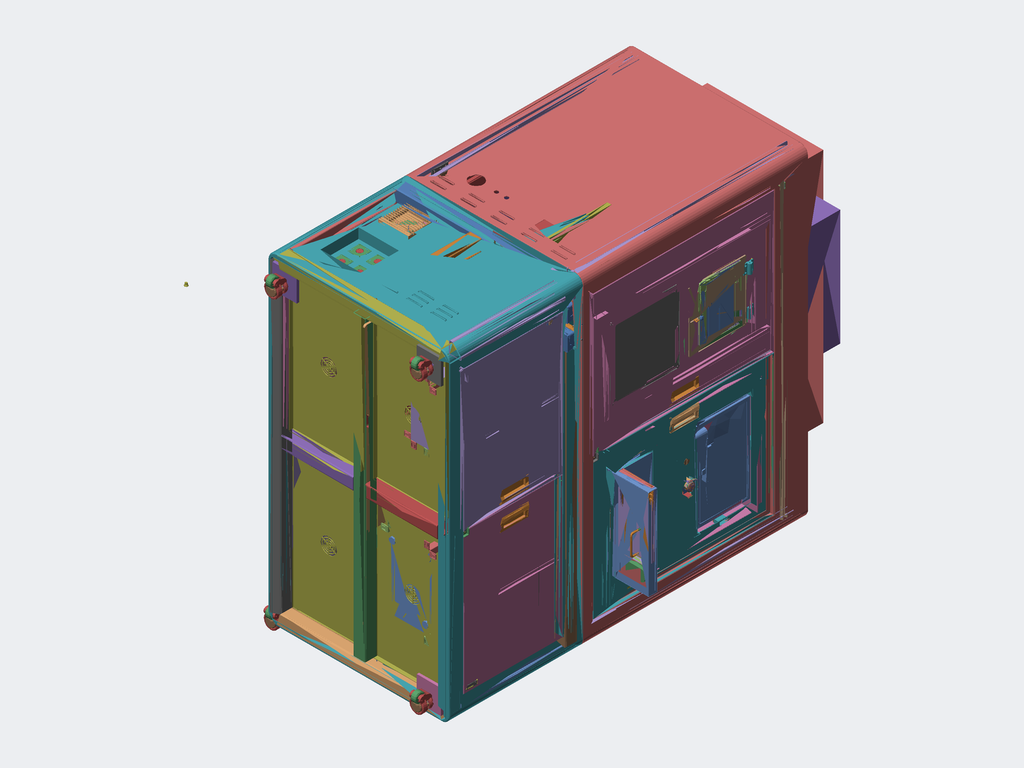Assembly | STEP file | 352 different items | 674 placed
Parts list (item | name | quantity | parent item | size | volume), first 270 of 352 items:
1 | Square tube frame_default<as machined> | x1 | in Lower frame | 896 x 660 x 1596 mm | 13190775 mm3
2 | Lower seal plate | x4 | in Lower frame | 708 x 358 x 20 mm | 574512 mm3
3 | ND25021-01-JDKM-103-TL | x1 | in Lower frame | 1490 x 15 x 786 mm | 17159345 mm3
4 | H_ND24021-01-JG-103-TL | x1 | in Lower frame | 1300 x 10 x 480 mm | 6236216 mm3
5 | PC | x1 | in Industrial PC assembly | 380 x 205 x 480 mm | 36265912 mm3
6 | PClimit part | x4 | in Industrial PC assembly, UPSassembly | 58 x 58 x 53 mm | 11788 mm3
7 | PC限位件2 | x4 | in Industrial PC assembly, UPSassembly | 58 x 58 x 53 mm | 11788 mm3
8 | Lower frame door panel | x2 | in Lower机架DoorPlate 2 | 20 x 700 x 502 mm | 890062 mm3
9 | HI_HFG87-17-001(2)^HFG87-17(2)_Lower机架DoorPlate 2 | x2 | in HFG87-17(2)^Lower机架DoorPlate 2 | 21.5 x 9 x 60 mm | 2771 mm3
10 | HI_HFG87-17-002(2)^HFG87-17(2)_Lower机架DoorPlate 2 | x2 | in HFG87-17(2)^Lower机架DoorPlate 2 | 18 x 8 x 84 mm | 2771 mm3
11 | XAM35_A140 | x7 | in Lower机架DoorPlate 2, 8, ND22021-MA-C-111, CE-005 | 64 x 22.5 x 140 mm | 66990 mm3
12 | OP02-QR01-J618 | x10 | in Door suction with buffer_9 | 27 x 27 x 12 mm | 2284 mm3
13 | Rubber buffer pad | x10 | in Door suction with buffer_9 | 22 x 22 x 7 mm | 750.57 mm3
14 | NHXCC20-5.5 | x10 | in Door suction with buffer_9 | 20 x 20 x 5.5 mm | 1502 mm3
15 | Flat-head stainless hex socket screw_M5_8 | x10 | in Door suction with buffer_9 | 10 x 10 x 11.1 mm | 211.569 mm3
16 | NNX210 | x2 | in 8 | 20 x 700 x 502 mm | 889755 mm3
17 | HI_HFG87-17-001(2)^ HFG87-17(2)_Lower frame door panel | x2 | in HFG87-17(2)^Lower frame door panel | 21.5 x 9 x 60 mm | 2771 mm3
18 | HI_HFG87-17-002(2)^ HFG87-17(2)_Lower frame door panel | x2 | in HFG87-17(2)^Lower frame door panel | 18 x 8 x 84 mm | 2771 mm3
19 | B-002 | x1 | in Lower frame | 1610 x 665 x 900 mm | 5357504 mm3
20 | with guard(8 mounting holes M5 metric threaded holes) Fan-KM | x2 | in Cooling Fanassembly-KM | - | -
21 | Ventilation filter assembly-KM | x2 | in Cooling Fanassembly-KM | 149 x 149 x 28 mm | 126448 mm3
22 | 电源1 | x1 | in Power switch | 105 x 85 x 79 mm | 30351 mm3
23 | 电源2 | x1 | in Power switch | 61 x 20 x 2 mm | 2336 mm3
24 | 电源3 | x1 | in Power switch | - | -
25 | AC20D-02C-A_0_^气源二联件-SMC | x1 | in 气源二联件-SMC | 83.2 x 172.3 x 53.4 mm | 301660 mm3
26 | _HSV08 -slide | x1 | in HSV08 | 30 x 30 x 32.5 mm | 8449 mm3
27 | _HSV08 Body | x1 | in HSV08 | 21.939 x 19.4 x 58 mm | 11797 mm3
28 | PL1002 | x2 | in 气源二联件-SMC | 35.315 x 36 x 18 mm | 6237 mm3
29 | ISE30A-01-N-ML_0_^气源二联件-SMC | x1 | in 气源二联件-SMC | 30 x 30 x 60.1 mm | 24209 mm3
30 | 接头6 | x2 | in Lower frame | 60 x 60 x 1.5 mm | 5253 mm3
31 | Ethernet port | x1 | in 接头3 | 60 x 60 x 1.5 mm | 5226 mm3
32 | 接头2 | x3 | in Lower frame | 60 x 60 x 1.5 mm | 5261 mm3
33 | UPS | x1 | in UPSassembly | 275 x 90 x 240 mm | 5940000 mm3
34 | H_ND24021-01-JG-098-TL | x1 | in power cover plate | 600 x 5 x 180 mm | 537768 mm3
35 | H_ND24021-01-JG-096-TL | x4 | in power cover plate | 43 x 20 x 132 mm | 6992 mm3
36 | HAU61-M5-L15^power cover plate | x4 | in power cover plate | 20 x 19.896 x 23 mm | 3201 mm3
37 | JK-Aviation plug | x4 | in Lower frame | 60 x 60 x 1.5 mm | 5200 mm3
38 | H_ND24021-01-JG-032-SL | x2 | in Air source cover plate | 300 x 5 x 255 mm | 380407 mm3
39 | HAQ07-M5^Air source cover plate | x2 | in Air source cover plate | 17 x 15 x 17 mm | 1673 mm3
40 | H_ND24021-01-JG-029-BJ | x3 | in Air source cover plate | 25.5 x 30 x 17.5 mm | 1036 mm3
41 | H_ND24021-01-JG-036-SL | x3 | in Air source cover plate | 22 x 22 x 6 mm | 2228 mm3
42 | H_ND24033-01-063-TL | x7 | in Hinge mount block, ND25021-MA-B-01机架 | 50 x 12 x 17 mm | 9145 mm3
43 | Damping hinge | x7 | in Hinge mount block, ND25021-MA-B-01机架 | 47 x 19.5 x 48 mm | 19859 mm3
44 | switch | x1 | in Limit switch | 94 x 38 x 28 mm | 52689 mm3
45 | 开关-2 | x1 | in Limit switch | 20 x 8 x 20 mm | 1727 mm3
46 | 开关-3 | x1 | in Limit switch | 103 x 10 x 18 mm | 6512 mm3
47 | b-005 | x1 | in Top cover | 1610 x 1120 x 900 mm | 8822368 mm3
48 | b-013 | x4 | in Top cover | 1094 x 21.5 x 33 mm | 117521 mm3
49 | b-016 | x2 | in Top cover | 1500 x 16.5 x 23 mm | 116188 mm3
50 | b-017 | x1 | in Top cover | 890 x 21.5 x 33 mm | 91588 mm3
51 | b-015 | x1 | in Top cover | 890 x 21.5 x 33 mm | 91888 mm3
52 | b-018 | x2 | in Top cover | 1530 x 21.5 x 33 mm | 164519 mm3
53 | b-019 | x2 | in Top cover | 550 x 21.5 x 33 mm | 59097 mm3
54 | FFU | x1 | in FFUassembly | 575 x 275 x 575 mm | 82748500 mm3
55 | FFUfilter | x1 | in FFUassembly | 575 x 69 x 575 mm | 19842875 mm3
56 | ND22021-MA-C-111-BJ | x1 | in ND22021-MA-C-111 | 700 x 900 x 22 mm | 1108313 mm3
57 | b-007 | x1 | in ND22021-MA-C-111 | 360 x 5 x 340 mm | 610031 mm3
58 | 45gtee-01 | x4 | in 磁性开关01 | 11.5 x 21.5 x 70 mm | 3184 mm3
59 | GLS_M1 | x4 | in 磁性开关01 | 50 x 10 x 14 mm | 4964 mm3
60 | GLS_S1 | x4 | in 磁性开关02 | 50 x 14 x 14 mm | 5525 mm3
61 | 4R32456 | x4 | in 磁性开关02 | 16.5 x 37.5 x 70 mm | 4931 mm3
62 | 10-inch touch screen_default | x1 | in ND22021-MA-C-111 | - | -
63 | ND22002-MA-D-007 | x1 | in Touch screen cover | 300 x 5 x 285 mm | 425473 mm3
64 | HAQ07-M5^Touch screen cover | x1 | in Touch screen cover | 17 x 15 x 17 mm | 1673 mm3
65 | b-021 | x1 | in Touch screen cover | 26.5 x 30 x 17.5 mm | 1038 mm3
66 | NX21002-02-MA-J-002 | x1 | in ND22021-MA-C-111 | 500 x 320 x 50 mm | 341606 mm3
67 | MB-005 | x2 | in CE-005 | 700 x 900 x 20 mm | 1064714 mm3
68 | b-006 | x2 | in CE-005 | 340 x 5 x 640 mm | 1086031 mm3
69 | _AKQ01-G-Z-6279A-001-ZZ | x4 | in AKQ01-G-Z-6279A | 36.75 x 12.05 x 79 mm | 10360 mm3
70 | _AKQ01-G-Z-6279A-002-ZZ | x4 | in AKQ01-G-Z-6279A | 7 x 7 x 82 mm | 3156 mm3
71 | _AKQ01-G-Z-6279A-003-ZZ | x4 | in AKQ01-G-Z-6279A | 36.75 x 12.05 x 79 mm | 10360 mm3
72 | AKB31 | x4 | in CE-005 | 53.5 x 14 x 24.5 mm | 11728 mm3
73 | NX21001-08-MA-02-003-001-DM2r | x1 | in NX21001-08-MA-J-02-003-DM2r | 900 x 700 x 54 mm | 1485136 mm3
74 | 3Dcax_LA39-B2-02Zr_20200421-DXDX-DB2r | x1 | in NX21001-08-MA-J-02-003-DM2r | - | -
75 | XAM35_A140r | x1 | in NX21001-08-MA-J-02-003-DM2r | 64 x 22.5 x 140 mm | 66990 mm3
76 | 键盘盒-01^TY.NE-0002-01-014A 键盘盒-dddeger | x2 | in TY.NE-0002-01-014A Keyboard box-dddeger | 464 x 43.4 x 183 mm | 167299 mm3
77 | 键盘盒-03^TY.NE-0002-01-014A 键盘盒-dddeger | x2 | in TY.NE-0002-01-014A Keyboard box-dddeger | 123.3 x 178.4 x 42.25 mm | 43523 mm3
78 | 键盘盒-05^TY.NE-0002-01-014A 键盘盒-dddeger | x2 | in TY.NE-0002-01-014A Keyboard box-dddeger | 100 x 24.8 x 10 mm | 3383 mm3
79 | 键盘盒-08^TY.NE-0002-01-014A 键盘盒-dddeger | x2 | in TY.NE-0002-01-014A Keyboard box-dddeger | 10 x 8 x 80 mm | 1580 mm3
80 | 键盘盒-08^TY.NE-0002-01-014A 键盘盒-dddeger | x2 | in TY.NE-0002-01-014A Keyboard box-dddeger | 10 x 8 x 80 mm | 1580 mm3
81 | HI_XAL51-D8-L100-H50-001^XAL51-D8-L100-H50 | x2 | in XAL51-D8-L100-H50 | 108 x 38 x 8 mm | 7383 mm3
82 | HI_XAL51-D8-L100-H50-002^XAL51-D8-L100-H50 | x4 | in XAL51-D8-L100-H50 | 8 x 22.5 x 8 mm | 786.148 mm3
83 | 鼠标盖Plate-01^TY.NE-0002-01-015A 鼠标盖Plate-dddeger | x2 | in TY.NE-0002-01-015A Mouse cover plate-dddeger | 121 x 15 x 138 mm | 25843 mm3
84 | TYLJ-BJ-007 Pin(1mm thick)-dddeger | x2 | in TY.NE-0002-01-015A Mouse cover plate-dddeger | 10 x 11 x 10 mm | 236.295 mm3
85 | CL225-3-Z Shengjiu spring plunger-dddeger | x2 | in TY.NE-0002-01-015A Mouse cover plate-dddeger | 24.6 x 87.5 x 9.2 mm | 4748 mm3
86 | TY.NE-0002-01-008A Mouse pad-dddeger | x2 | in TY.NE-0002-01-013A-A Keyboard box mount assembly-dddeger | 114 x 131 x 0.8 mm | 11930 mm3
87 | BMF01-A10 Yihe Da Magnet-dddeger | x2 | in TY.NE-0002-01-013A-A Keyboard box mount assembly-dddeger | 10.2 x 10 x 10 mm | 381.53 mm3
88 | TY.NE-0002-01-016A Keyboard tray-dddeger | x2 | in TY.NE-0002-01-013A-A Keyboard box mount assembly-dddeger | 323 x 27.127 x 169.984 mm | 77980 mm3
89 | TY.NE-0002-01-017A Keyboard press block-dddeger | x2 | in TY.NE-0002-01-013A-A Keyboard box mount assembly-dddeger | 220 x 22 x 1 mm | 4800 mm3
90 | T2x15x8 Rubber strip-dddeger_compressed | x4 | in TY.NE-0002-01-013A-A Keyboard box mount assembly-dddeger | 8 x 15 x 1.5 mm | 180 mm3
91 | Shuangfeiyankeyboard-FK112r | x2 | in TY.NE-0002-01-013A-A Keyboard box mount assembly-dddeger | 314 x 171 x 25.65 mm | 812761 mm3
92 | Shuangfeiyanmouse-OP-520NU2r | x2 | in TY.NE-0002-01-013A-A Keyboard box mount assembly-dddeger | 57 x 151 x 34.996 mm | 178729 mm3
93 | Rubber buffer padr | x4 | in Round magnetic catchr, Door suction with buffer_9r | 22 x 22 x 7 mm | 750.57 mm3
94 | NHXCC20-5.5r | x4 | in Round magnetic catchr, Door suction with buffer_9r | 20 x 20 x 5.5 mm | 1502 mm3
95 | Flat-head stainless hex socket screw_M5_8r | x4 | in Round magnetic catchr, Door suction with buffer_9r | 10 x 10 x 11.1 mm | 211.569 mm3
96 | cover plate43r | x1 | in NX21001-08-MA-J-02-003-DM2r | 540 x 81.5 x 600 mm | 684567 mm3
97 | OP02-QR01-J618r | x2 | in Door suction with buffer_9r | 27 x 27 x 12 mm | 2284 mm3
98 | Card reader | x1 | in NX21001-08-MA-J-02-003-DM2r | 62 x 14 x 127 mm | 71225 mm3
99 | Card reader Clamp plate | x1 | in NX21001-08-MA-J-02-003-DM2r | 60 x 4.5 x 192 mm | 11570 mm3
100 | Clamp plate | x3 | in NX21001-08-MA-J-02-003-DM2r | 40 x 2 x 45 mm | 2760 mm3
101 | E1916H Dell LCD monitor-ddde3r | x1 | in NX21001-08-MA-J-02-003-DM2r | 445.5 x 266 x 52.76 mm | 3312642 mm3
102 | ND25021-08-JDKM-03-BJ | x1 | in NX21001-08-MA-J-02-003-DM2r | 28 x 40 x 12 mm | 1335 mm3
103 | 护Plate 2 | x2 | in Top cover | 73 x 93 x 73 mm | 22681 mm3
104 | 护Plate 1 | x2 | in Top cover | 73 x 93 x 73 mm | 22681 mm3
105 | 护Plate 3 | x1 | in Top cover | 100 x 2 x 100 mm | 19866 mm3
106 | DIZUO-1^M4Y_Top cover | x1 | in M4Y^Top cover | 74 x 9.5 x 73 mm | 25864 mm3
107 | USB port | x1 | in Top cover | 28 x 28 x 27.6 mm | 11145 mm3
108 | D4NS_1CF_CAP^D4NS_1CF_Laser guard | x2 | in D4NS_1CF^Laser guard | 18 x 3.8 x 10.4 mm | 386.227 mm3
109 | D4NS_1CF_BASE^D4NS_1CF_Laser guard | x2 | in D4NS_1CF^Laser guard | 31 x 75 x 31.5 mm | 57393 mm3
110 | D4NS_1CF_HEAD^D4NS_1CF_Laser guard | x2 | in D4NS_1CF^Laser guard | 30.5 x 29 x 30.5 mm | 19068 mm3
111 | D4DS_K2.step | x2 | in D4NS_1CF^Laser guard | 37 x 30 x 11.5 mm | 1352 mm3
112 | H_ND24021-JJ-05-02-BJ | x1 | in Top cover | 30 x 40 x 2 mm | 2287 mm3
113 | H_ND24021-JJ-05-01-BJ | x1 | in Top cover | 80 x 35 x 42 mm | 11748 mm3
114 | ND25021-09-JDKM-03-BJ | x8 | in Top cover | 43 x 93 x 30 mm | 11155 mm3
115 | 复件 Part 1^Upper罩 | x1 | in Top cover | 1175 x 575 x 235 mm | 158771875 mm3
116 | H_ND24021-JJ-05-01B-BJ | x1 | in Top cover | 80 x 35 x 42 mm | 11748 mm3
117 | H_ND24021-JJ-05-02B-BJ | x2 | in Top cover | 45 x 40 x 5 mm | 8480 mm3
118 | H_ND24021-JJ-05-02C-BJ | x1 | in Top cover | 45 x 42 x 5 mm | 9347 mm3
119 | 复件 复件  HAQ07-M5^复件 Assembly 2_ND25021-MA-B-01机架 | x1 | in 复件 Assembly 2^ND25021-MA-B-01机架 | 17 x 15 x 17 mm | 1673 mm3
120 | _CGR01-60-U-001_1 | x4 | in CGR01-60-U | 29 x 49 x 49 mm | 45485 mm3
121 | _CGR01-60-U-002_1 | x4 | in CGR01-60-U | 70 x 63 x 89.5 mm | 81661 mm3
122 | _CGR01-60-U-003_1 | x4 | in CGR01-60-U | 46 x 32.8 x 53.116 mm | 30584 mm3
123 | _CGR01-60-U-004_1 | x4 | in CGR01-60-U | 55 x 41.5 x 55 mm | 64973 mm3
124 | H_ND24021-01-JG-108-SL | x1 | in ND25021-MA-B-01机架 | 105 x 5 x 161 mm | 82990 mm3
125 | ND25021-01-JDKM-01-TL | x1 | in Mechanism mount assembly | 1460 x 20 x 200 mm | 5782865 mm3
126 | ND25021-01-JDKM-02-TL | x1 | in Mechanism mount assembly | 1460 x 20 x 480 mm | 11435283 mm3
127 | ND25021-01-JDKM-03-TL | x2 | in Mechanism mount assembly | 340 x 16 x 90 mm | 294921 mm3
128 | ND25021-01-JDKM-04-TL | x2 | in Mechanism mount assembly | 290 x 16 x 90 mm | 253250 mm3
129 | ND25021-01-JDKM-05-TL | x2 | in Mechanism mount assembly | 120 x 16 x 80 mm | 95084 mm3
130 | ND25021-01-JDKMJ-06-TL | x2 | in Idler roller assembly (direct encoder) | 35 x 162.5 x 35 mm | 83750 mm3
131 | ND25021-01-JDKM-01-GJ | x2 | in One-way housed bearing | 64 x 19 x 46 mm | 25181 mm3
132 | BAY6202ZZ-J^One-way housed bearing | x2 | in One-way housed bearing | 11 x 34.971 x 35 mm | 6760 mm3
133 | TBP51-35 | x2 | in One-way housed bearing | 37.8 x 36.681 x 1.5 mm | 416.093 mm3
134 | BLC01-B2-L8 | x2 | in One-way housed bearing | 8 x 2 x 2 mm | 30.283 mm3
135 | BLC03-B5-L12 | x2 | in One-way housed bearing | 5 x 5 x 12 mm | 273.175 mm3
136 | HI_BFU71-6202ZZ-L40-S15S1^BFU71-6202ZZ-L40-S15_Idler roller assembly (direct encoder) | x2 | in BFU71-6202ZZ-L40-S15^Idler roller assembly (direct encoder) | 67 x 67 x 40 mm | 28798 mm3
137 | HI_BAY6202ZZ^BFU71-6202ZZ-L40-S15_Idler roller assembly (direct encoder) | x4 | in BFU71-6202ZZ-L40-S15^Idler roller assembly (direct encoder) | 11 x 35 x 35 mm | 6855 mm3
138 | E-BKE52-M15-1.0 | x2 | in Idler roller assembly (direct encoder) | 25 x 25 x 8 mm | 2176 mm3
139 | GCPSW20-6-6 | x2 | in Idler roller assembly (direct encoder) | 20 x 28.6 x 20 mm | 8036 mm3
140 | ND25021-01-JDKM-08-TL | x2 | in Direct-coupled encoder mount assembly | 110 x 5 x 62 mm | 19151 mm3
141 | E6B2_CWZ6C | x2 | in Direct-coupled encoder mount assembly | 40 x 57.5 x 59 mm | 51344 mm3
142 | ND25021-01-JDKM-07-TL | x2 | in Direct-coupled encoder mount assembly | 110 x 5 x 62 mm | 31358 mm3
143 | ND25021-01-JDKM-09B-TL | x8 | in Direct-coupled encoder mount assembly | 12 x 56 x 12 mm | 6119 mm3
144 | ND25021-01-JDKM-01-BJ | x2 | in Idler roller assembly (direct encoder) | 65 x 114 x 113 mm | 45715 mm3
145 | _bearing_6202 | x4 | in BGFSZ6202ZZ-40-S15 | 11 x 35 x 35 mm | 8312 mm3
146 | _housing_bgfszb6202-40-15 | x2 | in BGFSZ6202ZZ-40-S15 | 40 x 66 x 66 mm | 27673 mm3
147 | _RRING-C-INT-35 | x4 | in BGFSZ6202ZZ-40-S15 | 1.5 x 34.915 x 37 mm | 417.813 mm3
148 | E2B_S08KS01_WP_C1_CLAMPING_NUT | x4 | in E2B_S08KS01_WP_C1 | 13 x 15.011 x 4 mm | 382.328 mm3
149 | ND25021-01-JDKM-02-BJ | x2 | in E2B_S08KS01_WP_C1 | 14 x 45 x 28.5 mm | 1603 mm3
150 | E2B_S08KS01_WP_C1_BASE | x2 | in E2B_S08KS01_WP_C1 | 8 x 8 x 52 mm | 1995 mm3
151 | RSR-PB107_grease_nipple_joint(2)^SRS15MUU-220LM-G10_Buffer motion shaft | x1 | in SRS15MUU-220LM-G10^Buffer motion shaft | 8.5 x 4.5 x 4.5 mm | 76.658 mm3
152 | RSR15M1V220201 Track^SRS15MUU-220LM-G10_Buffer motion shaft | x1 | in SRS15MUU-220LM-G10^Buffer motion shaft | 240 x 9.5 x 15 mm | 30095 mm3
153 | RSR15M1V1Slider(2)^SRS15MUU-220LM-G10_Buffer motion shaft | x1 | in SRS15MUU-220LM-G10^Buffer motion shaft | 38.9 x 12 x 32 mm | 11407 mm3
154 | ND25021-01-JDKM-10-TL | x1 | in Buffer motion shaft | 35 x 15 x 28 mm | 12116 mm3
155 | _TDB86-M6-L20-001 | x1 | in TDB86-M6-L20 | 10 x 26 x 11.392 mm | 1007 mm3
156 | _TDB86-M6-L20-002 | x1 | in TDB86-M6-L20 | 10 x 3.6 x 11.392 mm | 234.612 mm3
157 | ND25021-01-JDKM-11-TL | x1 | in Buffer motion shaft | 35 x 15 x 32 mm | 12641 mm3
158 | ND25021-01-JDKM-13C-SL | x1 | in Buffer shaft part | 20 x 70.5 x 18 mm | 12721 mm3
159 | ND25021-01-JDKM-14-TL | x6 | in Buffer shaft part, Non-stick guide roller, Guide roller, Tension roller | 27 x 3 x 27 mm | 1464 mm3
160 | BAY6902ZZ-SUS | x12 | in Buffer shaft part, Non-stick guide roller, Guide roller, Tension roller | 7 x 28 x 28 mm | 2423 mm3
161 | ND25021-01-JDKM-15-TL | x1 | in Buffer shaft part | 35 x 64.5 x 35 mm | 29610 mm3
162 | ND25021-01-JDKM-12-TL | x1 | in Buffer motion shaft | 58 x 14 x 40 mm | 20081 mm3
163 | RJ1007LU_0_^Buffer motion shaft | x1 | in Buffer motion shaft | 62.3 x 16.166 x 14 mm | 4876 mm3
164 | ND25021-01-JDKM-16-TL | x1 | in Motor mount assembly | 100 x 10 x 85 mm | 63653 mm3
165 | 22010150--1-SOLI00^MS1H1-40B30CB-A331Z_1_ASM_Motor mount assembly | x1 | in MS1H1-40B30CB-A331Z_1_ASM^Motor mount assembly | 5 x 5 x 16.5 mm | 372.42 mm3
166 | _1-SO-126050001^MS1H1-40B30CB-A331Z_1_ASM_Motor mount assembly | x1 | in MS1H1-40B30CB-A331Z_1_ASM^Motor mount assembly | 3.9 x 0.3 x 3.9 mm | 2.443 mm3
167 | _1-SO-516090001^MS1H1-40B30CB-A331Z_1_ASM_Motor mount assembly | x1 | in MS1H1-40B30CB-A331Z_1_ASM^Motor mount assembly | 22 x 12.1 x 18.036 mm | 1625 mm3
168 | _1-SO-96830001^MS1H1-40B30CB-A331Z_1_ASM_Motor mount assembly | x1 | in MS1H1-40B30CB-A331Z_1_ASM^Motor mount assembly | 13.65 x 12.4 x 11.458 mm | 348.147 mm3
169 | _1-SO-363640001^MS1H1-40B30CB-A331Z_1_ASM_Motor mount assembly | x1 | in MS1H1-40B30CB-A331Z_1_ASM^Motor mount assembly | 3.9 x 0.3 x 3.9 mm | 2.443 mm3
170 | 31090521--MS1H1-400001^MS1H1-40B30CB-A331Z_1_ASM_Motor mount assembly | x1 | in MS1H1-40B30CB-A331Z_1_ASM^Motor mount assembly | 60 x 60 x 60 mm | 186186 mm3
171 | _1-SO-4430001^MS1H1-40B30CB-A331Z_1_ASM_Motor mount assembly | x1 | in MS1H1-40B30CB-A331Z_1_ASM^Motor mount assembly | 3.5 x 13.4 x 3.5 mm | 43.083 mm3
172 | _1-SO-265310001^MS1H1-40B30CB-A331Z_1_ASM_Motor mount assembly | x1 | in MS1H1-40B30CB-A331Z_1_ASM^Motor mount assembly | 14.371 x 12.4 x 12.872 mm | 348.152 mm3
173 | _1-SO-80980001^MS1H1-40B30CB-A331Z_1_ASM_Motor mount assembly | x1 | in MS1H1-40B30CB-A331Z_1_ASM^Motor mount assembly | 3.1 x 0.5 x 3.1 mm | 1.979 mm3
174 | _1-SO-150990001^MS1H1-40B30CB-A331Z_1_ASM_Motor mount assembly | x1 | in MS1H1-40B30CB-A331Z_1_ASM^Motor mount assembly | 3.1 x 0.5 x 3.1 mm | 1.979 mm3
175 | _1-SO-249010001^MS1H1-40B30CB-A331Z_1_ASM_Motor mount assembly | x1 | in MS1H1-40B30CB-A331Z_1_ASM^Motor mount assembly | 3.9 x 0.3 x 3.9 mm | 2.443 mm3
176 | _1-SO-416960001^MS1H1-40B30CB-A331Z_1_ASM_Motor mount assembly | x1 | in MS1H1-40B30CB-A331Z_1_ASM^Motor mount assembly | 30.6 x 11.855 x 32.912 mm | 2757 mm3
177 | _1-SO-486060001^MS1H1-40B30CB-A331Z_1_ASM_Motor mount assembly | x1 | in MS1H1-40B30CB-A331Z_1_ASM^Motor mount assembly | 3.5 x 13.4 x 3.5 mm | 43.083 mm3
178 | _1-SO-195900001^MS1H1-40B30CB-A331Z_1_ASM_Motor mount assembly | x1 | in MS1H1-40B30CB-A331Z_1_ASM^Motor mount assembly | 3.1 x 0.5 x 3.1 mm | 1.979 mm3
179 | _1-SO-318930001^MS1H1-40B30CB-A331Z_1_ASM_Motor mount assembly | x1 | in MS1H1-40B30CB-A331Z_1_ASM^Motor mount assembly | 3.5 x 13.4 x 3.5 mm | 43.083 mm3
180 | _60-1-SO0001^MS1H1-40B30CB-A331Z_1_ASM_Motor mount assembly | x1 | in MS1H1-40B30CB-A331Z_1_ASM^Motor mount assembly | 14.3 x 14.3 x 31.6 mm | 4477 mm3
181 | _1-SO-474100001^MS1H1-40B30CB-A331Z_1_ASM_Motor mount assembly | x1 | in MS1H1-40B30CB-A331Z_1_ASM^Motor mount assembly | 3.5 x 13.4 x 3.5 mm | 43.083 mm3
182 | _1-SO-642560001^MS1H1-40B30CB-A331Z_1_ASM_Motor mount assembly | x1 | in MS1H1-40B30CB-A331Z_1_ASM^Motor mount assembly | 3.9 x 0.3 x 3.9 mm | 2.443 mm3
183 | 31100246--1-SOLI00^MS1H1-40B30CB-A331Z_1_ASM_Motor mount assembly | x1 | in MS1H1-40B30CB-A331Z_1_ASM^Motor mount assembly | 60 x 62 x 17.5 mm | 52728 mm3
184 | _1-SO-753160001^MS1H1-40B30CB-A331Z_1_ASM_Motor mount assembly | x1 | in MS1H1-40B30CB-A331Z_1_ASM^Motor mount assembly | 3.1 x 0.5 x 3.1 mm | 1.979 mm3
185 | 30^MS1H1-40B30CB-A331Z_1_ASM_Motor mount assembly | x1 | in MS1H1-40B30CB-A331Z_1_ASM^Motor mount assembly | 30.6 x 7.2 x 22.8 mm | 1932 mm3
186 | 31090648--1-SOL000^MS1H1-40B30CB-A331Z_1_ASM_Motor mount assembly | x1 | in MS1H1-40B30CB-A331Z_1_ASM^Motor mount assembly | 60 x 60 x 4 mm | 12414 mm3
187 | 31900522--1-SOL000^MS1H1-40B30CB-A331Z_1_ASM_Motor mount assembly | x1 | in MS1H1-40B30CB-A331Z_1_ASM^Motor mount assembly | 60 x 60 x 12.5 mm | 36244 mm3
188 | 31740004--1-SOLI00^MS1H1-40B30CB-A331Z_1_ASM_Motor mount assembly | x1 | in MS1H1-40B30CB-A331Z_1_ASM^Motor mount assembly | 25 x 25 x 4 mm | 622.96 mm3
189 | ND25021-01-JDKM-17-TL | x4 | in Motor mount assembly | 15 x 54 x 15 mm | 9140 mm3
190 | ND25021-01-JDKM-19-TL | x1 | in Motor mount assembly | 14 x 12 x 100 mm | 14792 mm3
191 | TAD01-M6-L30^Motor mount assembly | x2 | in Motor mount assembly | 10 x 10 x 36 mm | 1238 mm3
192 | TAF02-M6-L40^Motor mount assembly | x1 | in Motor mount assembly | 10 x 10 x 44 mm | 1396 mm3
193 | ND25021-01-JDKM-18-TL | x1 | in Motor mount assembly | 100 x 12 x 118 mm | 133882 mm3
194 | C-HTPA25S5M150-A-N14^Pull-feed drive assembly | x1 | in Pull-feed drive assembly | 22 x 45 x 45 mm | 20511 mm3
195 | ND25021-01-JDKM-03B-TL | x4 | in Non-stick guide roller, Guide roller | 44 x 97 x 44 mm | 30962 mm3
196 | ND25021-01-JDKM-69-TL | x1 | in Non-stick guide roller | 40 x 68 x 40 mm | 54890 mm3
197 | BFU-2-42(2)^BFU71-6004ZZ-L55-S20_Drive roller assembly | x2 | in BFU71-6004ZZ-L55-S20^Drive roller assembly | 45.5 x 44.807 x 1.75 mm | 744.242 mm3
198 | BAY6004ZZ-bfu61_86-2(2)^BFU71-6004ZZ-L55-S20_Drive roller assembly | x2 | in BFU71-6004ZZ-L55-S20^Drive roller assembly | 12 x 42 x 42 mm | 10321 mm3
199 | BFU71-6004ZZ-L55-S20-001^BFU71-6004ZZ-L55-S20_Drive roller assembly | x1 | in BFU71-6004ZZ-L55-S20^Drive roller assembly | 77 x 77 x 55 mm | 52767 mm3
200 | C-HTPA25S5M150-A-N14^Drive roller assembly | x1 | in Drive roller assembly | 22 x 45 x 45 mm | 20511 mm3
201 | _RRING-C-INT-42 | x2 | in BGFSZ6004ZZ-55-S20 | 1.75 x 42.01 x 44.5 mm | 669.744 mm3
202 | _housing_bgfszb6004-55-22 | x1 | in BGFSZ6004ZZ-55-S20 | 55 x 77 x 77 mm | 52579 mm3
203 | _bearing_6004 | x2 | in BGFSZ6004ZZ-55-S20 | 12 x 42 x 42 mm | 12380 mm3
204 | BKN51-M20^Drive roller assembly | x1 | in Drive roller assembly | 37 x 32.043 x 11 mm | 4769 mm3
205 | ND25021-01-JDKM-02-GJ | x1 | in Drive roller assembly | 40 x 185 x 40 mm | 137740 mm3
206 | C-HTBN370S5M-150 | x1 | in Buffer shaft | 166.79 x 43.79 x 15 mm | 11319 mm3
207 | ND25021-01-JDKM-70-TL | x3 | in Guide roller | 40 x 68 x 40 mm | 54890 mm3
208 | ND25021-01-JDKM-22-TL | x1 | in Tension roller | 40 x 61 x 40 mm | 48754 mm3
209 | ND25021-01-JDKM-07-GJ | x1 | in Tension roller | 23 x 79 x 23 mm | 16613 mm3
210 | ND25021-01-JDKM-24-TL | x1 | in Tension control | 140 x 35 x 120 mm | 469712 mm3
211 | Wire connector | x1 | in Tension control | 14 x 27 x 37 mm | 6425 mm3
212 | CLT-50(20220226) | x1 | in Tension control | 69 x 104 x 104 mm | 248034 mm3
213 | ND25021-01-JDKM-09-GJ | x3 | in Clamp mount assembly, Clamp mount assembly 2 | 12 x 87 x 12 mm | 9716 mm3
214 | ND25021-01-JDKM-08-GJ | x10 | in Clamp mount assembly, Clamp mount assembly 2, Clamp rubber wheel | 20 x 5.9 x 20 mm | 1143 mm3
215 | ND25021-01-JDKM-25-TL | x3 | in Clamp mount assembly, Clamp mount assembly 2 | 75.5 x 12 x 50 mm | 42202 mm3
216 | ND25021-01-JDKM-26-TL | x2 | in Clamp mount assembly | 75.5 x 16 x 50 mm | 46652 mm3
217 | ND25021-01-JDKM-27-TL | x3 | in Clamp mount assembly, Clamp mount assembly 2 | 60 x 10 x 19 mm | 9293 mm3
218 | ND25021-01-JDKM-53-TL | x2 | in Clamp mount assembly | 46 x 12 x 50 mm | 25274 mm3
219 | Copy of QAF43-D50-d12-L50-T5^Clamp mount assembly | x2 | in Clamp mount assembly | 50 x 50 x 50 mm | 80359 mm3
220 | RSR15M1V160201 Track^SRS15MUU-160LM-G20_Pay-off clamp assembly | x1 | in SRS15MUU-160LM-G20^Pay-off clamp assembly | 160 x 9.5 x 15 mm | 20064 mm3
221 | RSR15M1V1Slider^SRS15MUU-160LM-G20_Pay-off clamp assembly | x1 | in SRS15MUU-160LM-G20^Pay-off clamp assembly | 38.9 x 12 x 32 mm | 11407 mm3
222 | RSR-PB107_grease_nipple_joint^SRS15MUU-160LM-G20_Pay-off clamp assembly | x1 | in SRS15MUU-160LM-G20^Pay-off clamp assembly | 8.5 x 4.5 x 4.5 mm | 76.658 mm3
223 | ND25021-01-JDKM-28-TL | x1 | in Pay-off clamp assembly | 95 x 16 x 50 mm | 64378 mm3
224 | CDM2L20-75Z_0_0_0_^Clamp cylinder assembly | x1 | in Clamp cylinder assembly | 191 x 40.011 x 55 mm | 57605 mm3
225 | F-M8X125F^Clamp cylinder assembly | x1 | in Clamp cylinder assembly | 24 x 24 x 51 mm | 10528 mm3
226 | ND25021-01-JDKM-31-TL | x1 | in Pay-off clamp assembly | 35 x 12 x 15 mm | 5586 mm3
227 | ND25021-01-JDKM-29-TL | x1 | in Pay-off clamp assembly | 90 x 12 x 40 mm | 41668 mm3
228 | ND25021-01-JDKM-30-TL | x1 | in Pay-off clamp assembly | 38 x 10 x 52 mm | 11845 mm3
229 | Pay-off roll | x1 | in Coding mechanism | 345.65 x 40 x 1390 mm | 521219 mm3
230 | Take-up roll | x1 | in Coding mechanism | 150 x 30 x 150 mm | 386793 mm3
231 | ND25021-01-JDKM-10-GJ | x1 | in Material sensor assembly | 38 x 90 x 38 mm | 19721 mm3
232 | ND25021-01-JDKM-32-TL | x1 | in Material sensor assembly | 65 x 15 x 26 mm | 22080 mm3
233 | ND25021-01-JDKM-11-BJ | x1 | in Material sensor assembly | 22 x 36 x 22 mm | 2627 mm3
234 | E3Z_D61-2M^Material sensor assembly | x1 | in Material sensor assembly | 124.985 x 38.085 x 10.8 mm | 16884 mm3
235 | E32-T11N 2M(欧姆龙280mm) | x2 | in Roll-diameter alarm sensor | 7 x 14.7 x 26.062 mm | 350.96 mm3
236 | ND25021-01-JDKM-03-BJ | x2 | in Roll-diameter alarm sensor | 102 x 33 x 17 mm | 5133 mm3
237 | APT8.024.0682 | x5 | in 3Dcax_XK-A1-Y2 | 73 x 73 x 37.5 mm | 72648 mm3
238 | APT8.315.0972 | x5 | in 3Dcax_XK-A1-Y2 | 72.5 x 72.5 x 22.5 mm | 32047 mm3
239 | 3Dcax_LA39-B2-20-y2 | x3 | in Manual start button box | 38.988 x 32.08 x 66.8 mm | 45407 mm3
240 | 3Dcax_LA39-B2-02Zr_20200421-DXDX-DB | x2 | in Emergency stop button | - | -
241 | ND25021-01-JDKM-01-SL | x2 | in Tension control panel | 200 x 175 x 5 mm | 174446 mm3
242 | TCN-002 Tension cont roller^Tension control panel | x2 | in Tension control panel | 83 x 120 x 166 mm | 1448834 mm3
243 | DTC13-Tension control panel-Taimake | x2 | in Tension control panel | 130 x 113 x 64.4 mm | 725565 mm3
244 | ND25021-01-JDKM-04-BJ | x2 | in Tension control panel | 200 x 175 x 100 mm | 153713 mm3
245 | ND25021-01-JDKM-36-TL | x1 | in Scanner moving assembly | 60 x 25 x 25 mm | 29527 mm3
246 | ND25021-01-JDKM-05-BJ | x1 | in Scanner moving assembly | 53 x 38 x 43 mm | 9223 mm3
247 | ND25021-01-JDKM-35-TL | x1 | in Scanner moving assembly | 55 x 20 x 50 mm | 28654 mm3
248 | ND25021-01-JDKM-21-GJ | x2 | in Scanner moving assembly | 12 x 180 x 12 mm | 20348 mm3
249 | MXQ8-50BT | x1 | in Scanner moving assembly | 37 x 25 x 155.8 mm | 80767 mm3
250 | ND25021-01-JDKM-34-TL | x1 | in Scanner moving assembly | 75 x 12 x 40 mm | 29872 mm3
251 | ND25021-01-JDKM-33-TL | x1 | in Scanner moving assembly | 103 x 12 x 50 mm | 59942 mm3
252 | sr-x100^Scanner moving assembly | x1 | in Scanner moving assembly | 37.2 x 188.7 x 73.89 mm | 134678 mm3
253 | ND25021-01-JDKM-38-TL | x1 | in Scanner moving assembly | 60 x 38 x 20 mm | 38918 mm3
254 | IR1020-01BG-A_0_^Coding mechanism | x1 | in Coding mechanism | 42 x 95.7 x 68.5 mm | 83604 mm3
255 | Mounting plate | x1 | in 激光Component 2 | 385 x 10 x 220 mm | 838731 mm3
256 | 连接Plate 3 | x1 | in 大族激光器5W紫外 | 60 x 10 x 63 mm | 19150 mm3
257 | 族光1号紫外激光器三维模型图202110 | x1 | in 大族激光器5W紫外 | 392.5 x 160 x 136 mm | 7837982 mm3
258 | 连接Plate 1 | x1 | in 大族激光器5W紫外 | 115.5 x 76 x 10 mm | 76508 mm3
259 | 连接Plate 2 | x1 | in 大族激光器5W紫外 | 56 x 56 x 65.079 mm | 55529 mm3
260 | 10A 模型图^大族激光器5W紫外 | x1 | in 大族激光器5W紫外 | - | -
261 | NJSL-802 SL-355-110-160-D10-LP[3D](2)^大族激光器5W紫外 | x1 | in 大族激光器5W紫外 | - | -
262 | 170升降-800mm立柱 | x1 | in 激光Component 2 | 425 x 361 x 928 mm | 5606632 mm3
263 | Scale ruler | x1 | in 激光Component 2 | 12 x 1 x 420 mm | 4971 mm3
264 | Pointer | x1 | in 激光Component 2 | 40 x 20 x 14.5 mm | 927.737 mm3
265 | HI_BAY6205ZZ^BFU71-6205ZZ-L55-S20_Mechanical tensioner (pay-off) | x2 | in BFU71-6205ZZ-L55-S20^Mechanical tensioner (pay-off) | 15 x 52 x 52 mm | 19388 mm3
266 | HI_BFU71-6205ZZ-L55-S20S1^BFU71-6205ZZ-L55-S20_Mechanical tensioner (pay-off) | x1 | in BFU71-6205ZZ-L55-S20^Mechanical tensioner (pay-off) | 95 x 95 x 55 mm | 71824 mm3
267 | ND25021-01-JDKM-40-TL | x4 | in Cylinder clamp assembly | 15 x 97 x 15 mm | 16574 mm3
268 | ND25021-01-JDKM-39-TL | x1 | in Cylinder clamp assembly | 106 x 12 x 106 mm | 126295 mm3
269 | PTL6M5A | x2 | in Cylinder clamp assembly | 24.696 x 29.5 x 11.7 mm | 2289 mm3
270 | CDQ2B32-15DZ-M9NL-XC8_0_XC8_0_^Cylinder clamp assembly | x1 | in Cylinder clamp assembly | 118.5 x 49.5 x 45 mm | 100397 mm3
Placements (level | parent | child | x y z in mm | rotation matrix by rows), first 173 of 831 lines:
1 | subassembly 2 | ND25021-MA-B-01机架 | -228.484 -655.603 993.897 | 1 0 0 0 1 0 0 0 1
2 | ND25021-MA-B-01机架 | Lower frame | -78.347 -11.05 943.448 | 1 0 0 0 1 0 0 0 1
3 | Lower frame | Square tube frame_default<as machined> | 174.375 -346.371 1175.0 | 1 0 0 0 1 0 0 0 1
3 | Lower frame | Lower seal plate | -273.625 -318.371 1145.0 | 0 -1 0 0 0 1 -1 0 0
3 | Lower frame | Lower seal plate | 144.375 -318.371 377.0 | 0 -1 0 0 0 1 -1 0 0
3 | Lower frame | Lower seal plate | 144.375 -318.371 1145.0 | 0 -1 0 0 0 1 -1 0 0
3 | Lower frame | Lower seal plate | -273.625 -318.371 377.0 | 0 -1 0 0 0 1 -1 0 0
3 | Lower frame | ND25021-01-JDKM-103-TL | -243.625 271.629 407.0 | 0 0 1 0 1 0 -1 0 0
3 | Lower frame | H_ND24021-01-JG-103-TL | -278.625 -76.371 407.0 | 0 -1 0 0 0 -1 1 0 0
3 | Lower frame | Industrial PC assembly | -35.0 5.0 -81.0 | 1 0 0 0 1 0 0 0 1
4 | Industrial PC assembly | PC | -23.125 -73.871 140.0 | 0 1 0 0 0 -1 -1 0 -0
4 | Industrial PC assembly | PClimit part | 80.375 -318.371 -50.0 | -1 0 0 0 0 1 0 1 0
4 | Industrial PC assembly | PClimit part | -126.625 -318.371 330.0 | 1 0 0 0 0 1 0 -1 0
4 | Industrial PC assembly | PC限位件2 | 79.375 -318.371 330.0 | 0 -1 0 0 0 1 -1 0 0
4 | Industrial PC assembly | PC限位件2 | -125.625 -318.371 -50.0 | 0 1 0 0 0 1 1 0 0
3 | Lower frame | Lower机架DoorPlate 2 | -894.507 257.511 -103.286 | -1 0 0 0 0 -1 0 -1 -0
4 | Lower机架DoorPlate 2 | Lower frame door panel | -220.882 -160.286 316.882 | 1 0 0 0 1 0 0 0 1
4 | Lower机架DoorPlate 2 | HFG87-17(2)^Lower机架DoorPlate 2 | -207.382 179.714 135.882 | 0 -1 0 -1 0 0 0 0 -1
5 | HFG87-17(2)^Lower机架DoorPlate 2 | HI_HFG87-17-001(2)^HFG87-17(2)_Lower机架DoorPlate 2 | -0.0 -0.0 -0.0 | 1 0 0 0 1 0 0 0 1
5 | HFG87-17(2)^Lower机架DoorPlate 2 | HI_HFG87-17-002(2)^HFG87-17(2)_Lower机架DoorPlate 2 | -0.0 -0.0 -0.0 | 1 0 0 0 1 0 0 0 1
4 | Lower机架DoorPlate 2 | XAM35_A140 | -210.882 -451.286 316.882 | 0 1 0 -1 0 0 0 0 1
4 | Lower机架DoorPlate 2 | Door suction with buffer_9 | -212.882 -494.786 547.382 | 0 0 1 1 0 0 0 1 -0
5 | Door suction with buffer_9 | OP02-QR01-J618 | -0.0 -0.0 -0.0 | 1 0 0 0 1 0 0 0 1
5 | Door suction with buffer_9 | Rubber buffer pad | -0.0 -0.0 -2.0 | -0.8873 -0.4612 0 -0.4612 0.8873 0 0 0 -1
5 | Door suction with buffer_9 | NHXCC20-5.5 | 0.0 -0.0 -5.75 | -0.9565 0.2917 0 0.2917 0.9565 0 0 0 -1
5 | Door suction with buffer_9 | Flat-head stainless hex socket screw_M5_8 | -0.0 -0.0 -4.95 | -0.6082 -0.7938 0 -0.7938 0.6082 0 0 0 -1
4 | Lower机架DoorPlate 2 | Door suction with buffer_9 | -212.882 -494.786 86.382 | 0 0 1 0 -1 0 1 0 -0
5 | Door suction with buffer_9 | OP02-QR01-J618 | -0.0 -0.0 -0.0 | 1 0 0 0 1 0 0 0 1
5 | Door suction with buffer_9 | Rubber buffer pad | -0.0 -0.0 -2.0 | -0.8873 -0.4612 0 -0.4612 0.8873 0 0 0 -1
5 | Door suction with buffer_9 | NHXCC20-5.5 | 0.0 -0.0 -5.75 | -0.9565 0.2917 0 0.2917 0.9565 0 0 0 -1
5 | Door suction with buffer_9 | Flat-head stainless hex socket screw_M5_8 | -0.0 -0.0 -4.95 | -0.6082 -0.7938 0 -0.7938 0.6082 0 0 0 -1
3 | Lower frame | Lower机架DoorPlate 2 | 407.257 257.511 917.286 | 1 0 0 0 0 -1 0 1 -0
4 | Lower机架DoorPlate 2 | Lower frame door panel | -220.882 -160.286 316.882 | 1 0 0 0 1 0 0 0 1
4 | Lower机架DoorPlate 2 | HFG87-17(2)^Lower机架DoorPlate 2 | -207.382 179.714 135.882 | 0 -1 0 -1 0 0 0 0 -1
5 | HFG87-17(2)^Lower机架DoorPlate 2 | HI_HFG87-17-001(2)^HFG87-17(2)_Lower机架DoorPlate 2 | -0.0 -0.0 -0.0 | 1 0 0 0 1 0 0 0 1
5 | HFG87-17(2)^Lower机架DoorPlate 2 | HI_HFG87-17-002(2)^HFG87-17(2)_Lower机架DoorPlate 2 | -0.0 -0.0 -0.0 | 1 0 0 0 1 0 0 0 1
4 | Lower机架DoorPlate 2 | XAM35_A140 | -210.882 -451.286 316.882 | 0 1 0 -1 0 0 0 0 1
4 | Lower机架DoorPlate 2 | Door suction with buffer_9 | -212.882 -494.786 547.382 | 0 0 1 1 0 0 0 1 -0
5 | Door suction with buffer_9 | OP02-QR01-J618 | -0.0 -0.0 -0.0 | 1 0 0 0 1 0 0 0 1
5 | Door suction with buffer_9 | Rubber buffer pad | -0.0 -0.0 -2.0 | -0.8873 -0.4612 0 -0.4612 0.8873 0 0 0 -1
5 | Door suction with buffer_9 | NHXCC20-5.5 | 0.0 -0.0 -5.75 | -0.9565 0.2917 0 0.2917 0.9565 0 0 0 -1
5 | Door suction with buffer_9 | Flat-head stainless hex socket screw_M5_8 | -0.0 -0.0 -4.95 | -0.6082 -0.7938 0 -0.7938 0.6082 0 0 0 -1
4 | Lower机架DoorPlate 2 | Door suction with buffer_9 | -212.882 -494.786 86.382 | 0 0 1 0 -1 0 1 0 -0
5 | Door suction with buffer_9 | OP02-QR01-J618 | -0.0 -0.0 -0.0 | 1 0 0 0 1 0 0 0 1
5 | Door suction with buffer_9 | Rubber buffer pad | -0.0 -0.0 -2.0 | -0.8873 -0.4612 0 -0.4612 0.8873 0 0 0 -1
5 | Door suction with buffer_9 | NHXCC20-5.5 | 0.0 -0.0 -5.75 | -0.9565 0.2917 0 0.2917 0.9565 0 0 0 -1
5 | Door suction with buffer_9 | Flat-head stainless hex socket screw_M5_8 | -0.0 -0.0 -4.95 | -0.6082 -0.7938 0 -0.7938 0.6082 0 0 0 -1
3 | Lower frame | Lower frame door panel | 407.257 -376.252 -103.286 | 1 0 0 0 0 1 0 -1 -0
4 | Lower frame door panel | NNX210 | -220.882 -160.286 316.882 | 1 0 0 0 1 0 0 0 1
4 | Lower frame door panel | HFG87-17(2)^Lower frame door panel | -207.382 179.714 135.882 | 0 -1 0 -1 0 0 0 0 -1
5 | HFG87-17(2)^Lower frame door panel | HI_HFG87-17-001(2)^ HFG87-17(2)_Lower frame door panel | -0.0 -0.0 -0.0 | 1 0 0 0 1 0 0 0 1
5 | HFG87-17(2)^Lower frame door panel | HI_HFG87-17-002(2)^ HFG87-17(2)_Lower frame door panel | -0.0 -0.0 -0.0 | 1 0 0 0 1 0 0 0 1
4 | Lower frame door panel | XAM35_A140 | -210.882 -451.286 316.882 | 0 1 0 -1 0 0 0 0 1
4 | Lower frame door panel | Door suction with buffer_9 | -212.882 -494.786 86.382 | 0 0 1 0 -1 0 1 0 -0
5 | Door suction with buffer_9 | OP02-QR01-J618 | -0.0 -0.0 -0.0 | 1 0 0 0 1 0 0 0 1
5 | Door suction with buffer_9 | Rubber buffer pad | -0.0 -0.0 -2.0 | -0.8873 -0.4612 0 -0.4612 0.8873 0 0 0 -1
5 | Door suction with buffer_9 | NHXCC20-5.5 | 0.0 -0.0 -5.75 | -0.9565 0.2917 0 0.2917 0.9565 0 0 0 -1
5 | Door suction with buffer_9 | Flat-head stainless hex socket screw_M5_8 | -0.0 -0.0 -4.95 | -0.6082 -0.7938 0 -0.7938 0.6082 0 0 0 -1
4 | Lower frame door panel | Door suction with buffer_9 | -212.882 -494.786 547.382 | 0 0 1 1 0 0 0 1 -0
5 | Door suction with buffer_9 | OP02-QR01-J618 | -0.0 -0.0 -0.0 | 1 0 0 0 1 0 0 0 1
5 | Door suction with buffer_9 | Rubber buffer pad | -0.0 -0.0 -2.0 | -0.8873 -0.4612 0 -0.4612 0.8873 0 0 0 -1
5 | Door suction with buffer_9 | NHXCC20-5.5 | 0.0 -0.0 -5.75 | -0.9565 0.2917 0 0.2917 0.9565 0 0 0 -1
5 | Door suction with buffer_9 | Flat-head stainless hex socket screw_M5_8 | -0.0 -0.0 -4.95 | -0.6082 -0.7938 0 -0.7938 0.6082 0 0 0 -1
3 | Lower frame | Lower frame door panel | -894.507 -376.252 917.286 | -1 0 0 0 0 1 0 1 0
4 | Lower frame door panel | NNX210 | -220.882 -160.286 316.882 | 1 0 0 0 1 0 0 0 1
4 | Lower frame door panel | HFG87-17(2)^Lower frame door panel | -207.382 179.714 135.882 | 0 -1 0 -1 0 0 0 0 -1
5 | HFG87-17(2)^Lower frame door panel | HI_HFG87-17-001(2)^ HFG87-17(2)_Lower frame door panel | -0.0 -0.0 -0.0 | 1 0 0 0 1 0 0 0 1
5 | HFG87-17(2)^Lower frame door panel | HI_HFG87-17-002(2)^ HFG87-17(2)_Lower frame door panel | -0.0 -0.0 -0.0 | 1 0 0 0 1 0 0 0 1
4 | Lower frame door panel | XAM35_A140 | -210.882 -451.286 316.882 | 0 1 0 -1 0 0 0 0 1
4 | Lower frame door panel | Door suction with buffer_9 | -212.882 -494.786 86.382 | 0 0 1 0 -1 0 1 0 -0
5 | Door suction with buffer_9 | OP02-QR01-J618 | -0.0 -0.0 -0.0 | 1 0 0 0 1 0 0 0 1
5 | Door suction with buffer_9 | Rubber buffer pad | -0.0 -0.0 -2.0 | -0.8873 -0.4612 0 -0.4612 0.8873 0 0 0 -1
5 | Door suction with buffer_9 | NHXCC20-5.5 | 0.0 -0.0 -5.75 | -0.9565 0.2917 0 0.2917 0.9565 0 0 0 -1
5 | Door suction with buffer_9 | Flat-head stainless hex socket screw_M5_8 | -0.0 -0.0 -4.95 | -0.6082 -0.7938 0 -0.7938 0.6082 0 0 0 -1
4 | Lower frame door panel | Door suction with buffer_9 | -212.882 -494.786 547.382 | 0 0 1 1 0 0 0 1 -0
5 | Door suction with buffer_9 | OP02-QR01-J618 | -0.0 -0.0 -0.0 | 1 0 0 0 1 0 0 0 1
5 | Door suction with buffer_9 | Rubber buffer pad | -0.0 -0.0 -2.0 | -0.8873 -0.4612 0 -0.4612 0.8873 0 0 0 -1
5 | Door suction with buffer_9 | NHXCC20-5.5 | 0.0 -0.0 -5.75 | -0.9565 0.2917 0 0.2917 0.9565 0 0 0 -1
5 | Door suction with buffer_9 | Flat-head stainless hex socket screw_M5_8 | -0.0 -0.0 -4.95 | -0.6082 -0.7938 0 -0.7938 0.6082 0 0 0 -1
3 | Lower frame | B-002 | -243.625 -45.871 407.0 | 0 0 -1 0 1 0 1 0 -0
3 | Lower frame | Cooling Fanassembly-KM | -453.049 85.95 614.711 | 0 1 0 -1 0 0 0 0 1
4 | Cooling Fanassembly-KM | with guard(8 mounting holes M5 metric threaded holes) Fan-KM | -1.929 -9.326 558.289 | 0 -1 0 -1 0 0 0 0 -1
4 | Cooling Fanassembly-KM | Ventilation filter assembly-KM | -1.929 -9.326 605.289 | 0 -1 0 -1 0 0 0 0 -1
3 | Lower frame | Cooling Fanassembly-KM | -474.201 -79.05 199.289 | 0 -1 0 -1 0 0 0 0 -1
4 | Cooling Fanassembly-KM | with guard(8 mounting holes M5 metric threaded holes) Fan-KM | -1.929 -9.326 558.289 | 0 -1 0 -1 0 0 0 0 -1
4 | Cooling Fanassembly-KM | Ventilation filter assembly-KM | -1.929 -9.326 605.289 | 0 -1 0 -1 0 0 0 0 -1
3 | Lower frame | Power switch | -460.396 38.406 -250 | 0 -1 0 -1 0 0 0 0 -1
4 | Power switch | 电源1 | -86.723 2.23 133 | 1 0 0 0 1 0 0 0 1
4 | Power switch | 电源2 | -86.723 -23.77 65.5 | 0 1 0 1 0 0 0 0 -1
4 | Power switch | 电源3 | -90.726 2.23 92.785 | 1 0 0 0 0 -1 0 1 0
3 | Lower frame | 气源二联件-SMC | -344.389 1.176 -588.273 | 0 0 1 0 1 0 -1 0 0
4 | 气源二联件-SMC | AC20D-02C-A_0_^气源二联件-SMC | -275.273 90.653 280.764 | 0 0 1 0 1 0 -1 0 0
4 | 气源二联件-SMC | HSV08 | -275.273 90.653 345.163 | -0.5 -0.866 0 -0.866 0.5 0 0 0 -1
5 | HSV08 | _HSV08 -slide | -0.0 0.0 -0.0 | 1 0 0 0 1 0 0 0 1
5 | HSV08 | _HSV08 Body | -0.0 0.0 -0.0 | 1 0 0 0 1 0 0 0 1
4 | 气源二联件-SMC | PL1002 | -275.273 90.653 365.764 | -1 0 0 0 0 1 0 1 0
4 | 气源二联件-SMC | PL1002 | -275.273 90.653 199.564 | -1 0 0 0 0 -1 0 -1 0
4 | 气源二联件-SMC | ISE30A-01-N-ML_0_^气源二联件-SMC | -245.273 90.653 280.764 | 0 0 1 0 1 0 -1 0 -0
3 | Lower frame | 接头6 | -63.625 -155.871 -343.75 | 1 0 0 0 1 0 0 0 1
3 | Lower frame | 接头3 | -216.137 -162.083 -283.75 | -1 0 0 0 1 0 0 0 -1
4 | 接头3 | Ethernet port | -67.512 6.213 60.0 | 1 0 0 0 1 0 0 0 1
3 | Lower frame | 接头2 | -148.625 -240.871 -343.75 | 1 0 0 0 1 0 0 0 1
3 | Lower frame | UPSassembly | -280.723 603.245 768.42 | 1 0 0 0 1 0 0 0 1
4 | UPSassembly | UPS | 280.097 -799.616 51.08 | 0 1 0 0 0 -1 -1 0 -0
4 | UPSassembly | PC限位件2 | 325.097 -916.616 188.58 | 0 -1 0 0 0 1 -1 0 0
4 | UPSassembly | PClimit part | 235.097 -916.616 188.58 | 1 0 0 0 0 1 0 -1 0
4 | UPSassembly | PC限位件2 | 235.097 -916.616 -86.42 | 0 1 0 0 0 1 1 0 0
4 | UPSassembly | PClimit part | 325.097 -916.616 -86.42 | -1 0 0 0 0 1 0 1 0
3 | Lower frame | power cover plate | -397.687 23.629 165.462 | 0 -1 0 0 0 -1 1 0 0
4 | power cover plate | H_ND24021-01-JG-098-TL | -73.462 17.938 -0.0 | 1 0 0 0 1 0 0 0 1
4 | power cover plate | H_ND24021-01-JG-096-TL | 186.538 -114.062 -80.0 | -1 0 0 0 0 -1 0 -1 0
4 | power cover plate | H_ND24021-01-JG-096-TL | 186.538 -114.062 80.0 | -1 0 0 0 0 -1 0 -1 0
4 | power cover plate | H_ND24021-01-JG-096-TL | -333.462 -114.062 80.0 | 1 0 0 0 0 -1 0 1 -0
4 | power cover plate | H_ND24021-01-JG-096-TL | -333.462 -114.062 -80.0 | 1 0 0 0 0 -1 0 1 -0
4 | power cover plate | HAU61-M5-L15^power cover plate | 176.538 22.938 80.0 | 0.1207 0.9927 0 0 0 -1 -0.9927 0.1207 0
4 | power cover plate | HAU61-M5-L15^power cover plate | 176.538 22.938 -80.0 | 0.1207 0.9927 0 0 0 -1 -0.9927 0.1207 0
4 | power cover plate | HAU61-M5-L15^power cover plate | -323.462 22.938 -80.0 | 0.1207 0.9927 0 0 0 -1 -0.9927 0.1207 0
4 | power cover plate | HAU61-M5-L15^power cover plate | -323.462 22.938 80.0 | 0.1207 0.9927 0 0 0 -1 -0.9927 0.1207 0
3 | Lower frame | JK-Aviation plug | -418.625 -198.371 1157.75 | -1 0 0 0 1 0 0 0 -1
3 | Lower frame | 接头6 | 21.375 -155.871 -343.75 | 1 0 0 0 1 0 0 0 1
3 | Lower frame | 接头2 | -63.625 -240.871 -343.75 | 1 0 0 0 1 0 0 0 1
3 | Lower frame | 接头2 | 21.375 -240.871 -343.75 | 1 0 0 0 1 0 0 0 1
3 | Lower frame | JK-Aviation plug | -418.625 -108.371 1157.75 | -1 0 0 0 1 0 0 0 -1
3 | Lower frame | JK-Aviation plug | -508.625 -108.371 1157.75 | -1 0 0 0 1 0 0 0 -1
3 | Lower frame | JK-Aviation plug | -508.625 -198.371 1157.75 | -1 0 0 0 1 0 0 0 -1
3 | Lower frame | Air source cover plate | -1564.001 -1025.445 -158.037 | 0 0 1 0 1 0 -1 0 -0
4 | Air source cover plate | H_ND24021-01-JG-032-SL | 241.963 1075.574 1500.376 | 0 1 0 0 0 -1 -1 0 0
4 | Air source cover plate | HAQ07-M5^Air source cover plate | 236.963 968.074 1530.376 | 0 1 0 0.8412 0 -0.5408 -0.5408 0 -0.8412
4 | Air source cover plate | H_ND24021-01-JG-029-BJ | 236.463 963.484 1501.126 | 1 0 0 0 -1 0 0 0 -1
4 | Air source cover plate | H_ND24021-01-JG-036-SL | 241.963 968.074 1470.376 | 0 0 -1 0.976 -0.2176 0 -0.2176 -0.976 -0
4 | Air source cover plate | Hinge mount block | 125.016 982.914 1420.693 | 0 1 0 0 0 -1 -1 0 -0
5 | Hinge mount block | H_ND24033-01-063-TL | 15.817 109.947 -241.66 | 1 0 0 0 1 0 0 0 1
5 | Hinge mount block | Damping hinge | 15.817 126.447 -226.16 | 1 0 0 0 -1 0 0 0 -1
4 | Air source cover plate | Hinge mount block | 125.016 982.914 1611.693 | 0 1 0 0 0 -1 -1 0 -0
5 | Hinge mount block | H_ND24033-01-063-TL | 15.817 109.947 -241.66 | 1 0 0 0 1 0 0 0 1
5 | Hinge mount block | Damping hinge | 15.817 126.447 -226.16 | 1 0 0 0 -1 0 0 0 -1
3 | Lower frame | Limit switch | -650.625 181.749 205.839 | 0 0 -1 0 -1 0 -1 0 -0
4 | Limit switch | switch | -61.161 15.12 -0.0 | 1 0 0 0 1 0 0 0 1
4 | Limit switch | 开关-2 | -102.161 49.12 0.0 | -0.4226 0 -0.9063 0 1 0 0.9063 0 -0.4226
4 | Limit switch | 开关-3 | -74.972 53.12 12.678 | 0.9063 0 -0.4226 0 1 0 0.4226 0 0.9063
2 | ND25021-MA-B-01机架 | Top cover | -1443.762 2883.468 3009.243 | 0.4169 0.9068 0.06165 0.0257 0.05604 -0.9981 -0.9086 0.4177 6e-05
3 | Top cover | b-005 | 1922.226 209.59 2113.051 | -0.9086 0.0257 -0.4169 0.4177 0.05604 -0.9068 6e-05 -0.9981 -0.06165
3 | Top cover | b-013 | 2487.083 -472.152 2100.34 | 0.0257 -0.9086 0.4169 0.05604 0.4177 0.9068 -0.9981 6e-05 0.06165
3 | Top cover | b-013 | 2806.879 223.394 2147.624 | 0.0257 -0.9086 0.4169 0.05604 0.4177 0.9068 -0.9981 6e-05 0.06165
3 | Top cover | b-013 | 1356.804 890.099 2147.719 | 0.0257 0.9086 -0.4169 0.05604 -0.4177 -0.9068 -0.9981 -6e-05 -0.06165
3 | Top cover | b-013 | 1037.008 194.554 2100.435 | 0.0257 0.9086 -0.4169 0.05604 -0.4177 -0.9068 -0.9981 -6e-05 -0.06165
3 | Top cover | b-016 | 2120.492 640.874 1695.018 | 0.9086 -0.4169 0.0257 -0.4177 -0.9068 0.05604 -6e-05 -0.06165 -0.9981
3 | Top cover | b-016 | 1746.909 -171.654 1639.782 | 0.9086 0.4169 -0.0257 -0.4177 0.9068 -0.05604 -6e-05 0.06165 0.9981
3 | Top cover | b-017 | 1226.52 567.318 1556.159 | 0.4169 -0.0257 0.9086 0.9068 -0.05604 -0.4177 0.06165 0.9981 -6e-05
3 | Top cover | b-015 | 2646.612 -85.602 1556.065 | 0.4169 -0.0257 0.9086 0.9068 -0.05604 -0.4177 0.06165 0.9981 -6e-05
3 | Top cover | b-018 | 1815.027 -23.485 1538.142 | 0.9086 -0.0257 -0.4169 -0.4177 -0.05604 -0.9068 -6e-05 0.9981 -0.06165
3 | Top cover | b-018 | 2058.105 505.202 1574.082 | 0.9086 -0.0257 -0.4169 -0.4177 -0.05604 -0.9068 -6e-05 0.9981 -0.06165
3 | Top cover | b-019 | 1399.148 487.949 1556.147 | -0.4169 -0.0257 -0.9086 -0.9068 -0.05604 0.4177 -0.06165 0.9981 6e-05
3 | Top cover | b-019 | 2473.984 -6.232 1556.077 | -0.4169 -0.0257 -0.9086 -0.9068 -0.05604 0.4177 -0.06165 0.9981 6e-05
3 | Top cover | FFUassembly | 1.131 2.466 -43.916 | 1 0 0 0 1 0 0 0 1
4 | FFUassembly | FFU | 1937.26 242.371 1529.163 | 0.9086 0.0257 0.4169 -0.4177 0.05604 0.9068 -6e-05 -0.9981 0.06165
4 | FFUassembly | FFUfilter | 1935.487 238.505 1598.032 | 0.9086 0.0257 0.4169 -0.4177 0.05604 0.9068 -6e-05 -0.9981 0.06165
3 | Top cover | ND22021-MA-C-111 | 1242.775 1682.219 2232.374 | -0.9086 0.0257 -0.4169 0.4177 0.05604 -0.9068 6e-05 -0.9981 -0.06165
4 | ND22021-MA-C-111 | ND22021-MA-C-111-BJ | -882.504 -5.963 611.0 | 1 0 0 0 1 0 0 0 1
4 | ND22021-MA-C-111 | b-007 | -882.504 -195.963 613.5 | -1 0 0 0 0 1 0 1 -0
4 | ND22021-MA-C-111 | XAM35_A140 | -1173.504 -5.963 619.5 | -1 0 0 0 0 -1 0 -1 -0
4 | ND22021-MA-C-111 | Door suction with buffer_9 | -1217.504 -440.963 621.0 | 1 0 0 0 -1 0 0 0 -1
5 | Door suction with buffer_9 | OP02-QR01-J618 | -0.0 -0.0 -0.0 | 1 0 0 0 1 0 0 0 1
5 | Door suction with buffer_9 | Rubber buffer pad | -0.0 -0.0 -2.0 | -0.8873 -0.4612 0 -0.4612 0.8873 0 0 0 -1
5 | Door suction with buffer_9 | NHXCC20-5.5 | 0.0 -0.0 -5.75 | -0.9565 0.2917 0 0.2917 0.9565 0 0 0 -1
5 | Door suction with buffer_9 | Flat-head stainless hex socket screw_M5_8 | -0.0 -0.0 -4.95 | -0.6082 -0.7938 0 -0.7938 0.6082 0 0 0 -1
4 | ND22021-MA-C-111 | Door suction with buffer_9 | -1217.504 429.037 621.0 | 0 -1 0 -1 0 0 0 0 -1
5 | Door suction with buffer_9 | OP02-QR01-J618 | -0.0 -0.0 -0.0 | 1 0 0 0 1 0 0 0 1
5 | Door suction with buffer_9 | Rubber buffer pad | -0.0 -0.0 -2.0 | -0.8873 -0.4612 0 -0.4612 0.8873 0 0 0 -1
5 | Door suction with buffer_9 | NHXCC20-5.5 | 0.0 -0.0 -5.75 | -0.9565 0.2917 0 0.2917 0.9565 0 0 0 -1
5 | Door suction with buffer_9 | Flat-head stainless hex socket screw_M5_8 | -0.0 -0.0 -4.95 | -0.6082 -0.7938 0 -0.7938 0.6082 0 0 0 -1
4 | ND22021-MA-C-111 | Magnetic switch | -1088.56 392.619 586.223 | -0.6204 0.291 0.7283 -0.1693 -0.9564 0.2379 0.7658 0.02433 0.6426
5 | Magnetic switch | 磁性开关01 | 1258.846 -497.07 -566.955 | 1 0 0 0 1 0 0 0 1